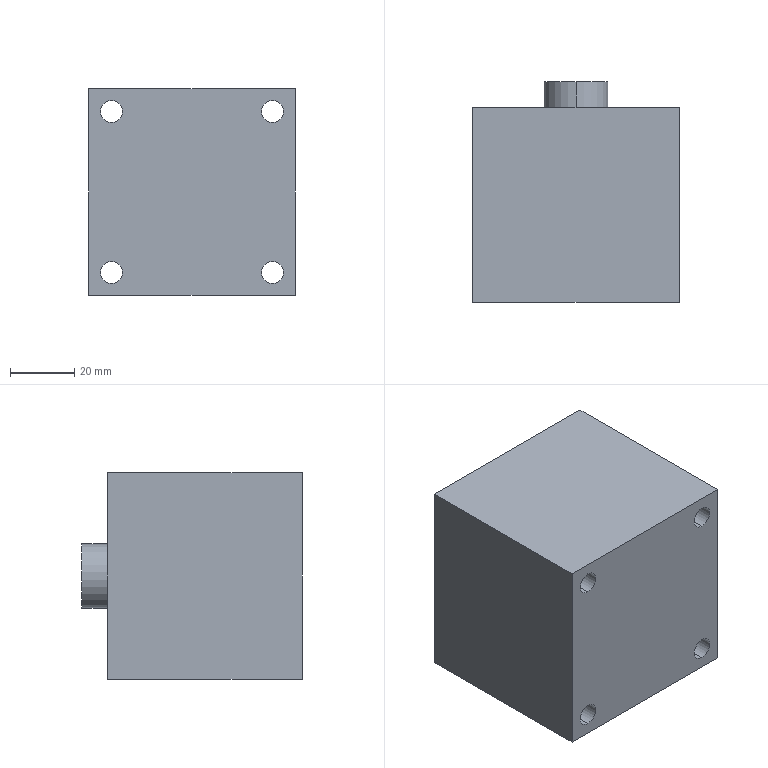Part | STEP file | 1 solid | 21 faces | box 64 x 68.5 x 64 mm | volume 240094 mm3 | cylinder 12 | plane 7 | cone 2 | commonest cylinder face diameters 6.8 x8 8.5 x2 20 x2
STEP:
#1=CARTESIAN_POINT('',(0.,0.,0.));
#2=DIRECTION('',(0.,0.,1.));
#3=DIRECTION('',(1.,0.,0.));
#4=AXIS2_PLACEMENT_3D('',#1,#2,#3);
#5=CARTESIAN_POINT('',(0.,44.,4.25));
#6=VERTEX_POINT('',#5);
#7=CARTESIAN_POINT('',(0.,68.5,4.25));
#8=VERTEX_POINT('',#7);
#9=CARTESIAN_POINT('',(0.,68.5,4.25));
#10=DIRECTION('',(0.,1.,0.));
#11=VECTOR('',#10,1.);
#12=LINE('',#9,#11);
#13=CARTESIAN_POINT('',(0.,68.5,0.));
#14=DIRECTION('',(0.,1.,0.));
#15=DIRECTION('',(0.,0.,1.));
#16=AXIS2_PLACEMENT_3D('',#13,#14,#15);
#17=CYLINDRICAL_SURFACE('',#16,4.25);
#18=CARTESIAN_POINT('',(6.283,0.));
#19=DIRECTION('',(0.,1.));
#20=VECTOR('',#19,1.);
#21=LINE('',#18,#20);
#22=(GEOMETRIC_REPRESENTATION_CONTEXT(2)PARAMETRIC_REPRESENTATION_CONTEXT()REPRESENTATION_CONTEXT('',''));
#23=DEFINITIONAL_REPRESENTATION('',(#21),#22);
#24=PCURVE('',#17,#23);
#25=CARTESIAN_POINT('',(0.,68.5,0.));
#26=DIRECTION('',(0.,1.,0.));
#27=DIRECTION('',(0.,0.,1.));
#28=AXIS2_PLACEMENT_3D('',#25,#26,#27);
#29=CYLINDRICAL_SURFACE('',#28,4.25);
#30=CARTESIAN_POINT('',(0.,0.));
#31=DIRECTION('',(0.,1.));
#32=VECTOR('',#31,1.);
#33=LINE('',#30,#32);
#34=(GEOMETRIC_REPRESENTATION_CONTEXT(2)PARAMETRIC_REPRESENTATION_CONTEXT()REPRESENTATION_CONTEXT('',''));
#35=DEFINITIONAL_REPRESENTATION('',(#33),#34);
#36=PCURVE('',#29,#35);
#37=SURFACE_CURVE('',#12,(#24,#36),.PCURVE_S1.);
#38=EDGE_CURVE('',#6,#8,#37,.T.);
#39=ORIENTED_EDGE('',*,*,#38,.T.);
#40=CARTESIAN_POINT('',(0.,68.5,-4.25));
#41=VERTEX_POINT('',#40);
#42=CARTESIAN_POINT('',(0.,68.5,0.));
#43=DIRECTION('',(0.,1.,0.));
#44=DIRECTION('',(0.,0.,1.));
#45=AXIS2_PLACEMENT_3D('',#42,#43,#44);
#46=CIRCLE('',#45,4.25);
#47=CARTESIAN_POINT('',(0.,0.));
#48=DIRECTION('',(1.,0.));
#49=VECTOR('',#48,1.);
#50=LINE('',#47,#49);
#51=(GEOMETRIC_REPRESENTATION_CONTEXT(2)PARAMETRIC_REPRESENTATION_CONTEXT()REPRESENTATION_CONTEXT('',''));
#52=DEFINITIONAL_REPRESENTATION('',(#50),#51);
#53=PCURVE('',#17,#52);
#54=CARTESIAN_POINT('',(0.,68.5,0.));
#55=DIRECTION('',(0.,1.,0.));
#56=DIRECTION('',(0.,0.,1.));
#57=AXIS2_PLACEMENT_3D('',#54,#55,#56);
#58=PLANE('',#57);
#59=CARTESIAN_POINT('',(0.,0.));
#60=DIRECTION('',(1.,0.));
#61=AXIS2_PLACEMENT_2D('',#59,#60);
#62=CIRCLE('',#61,4.25);
#63=(GEOMETRIC_REPRESENTATION_CONTEXT(2)PARAMETRIC_REPRESENTATION_CONTEXT()REPRESENTATION_CONTEXT('',''));
#64=DEFINITIONAL_REPRESENTATION('',(#62),#63);
#65=PCURVE('',#58,#64);
#66=SURFACE_CURVE('',#46,(#53,#65),.PCURVE_S1.);
#67=EDGE_CURVE('',#41,#8,#66,.T.);
#68=ORIENTED_EDGE('',*,*,#67,.F.);
#69=CARTESIAN_POINT('',(0.,44.,-4.25));
#70=VERTEX_POINT('',#69);
#71=CARTESIAN_POINT('',(0.,68.5,-4.25));
#72=DIRECTION('',(0.,1.,0.));
#73=VECTOR('',#72,1.);
#74=LINE('',#71,#73);
#75=CARTESIAN_POINT('',(3.142,0.));
#76=DIRECTION('',(0.,1.));
#77=VECTOR('',#76,1.);
#78=LINE('',#75,#77);
#79=(GEOMETRIC_REPRESENTATION_CONTEXT(2)PARAMETRIC_REPRESENTATION_CONTEXT()REPRESENTATION_CONTEXT('',''));
#80=DEFINITIONAL_REPRESENTATION('',(#78),#79);
#81=PCURVE('',#17,#80);
#82=CARTESIAN_POINT('',(3.142,0.));
#83=DIRECTION('',(0.,1.));
#84=VECTOR('',#83,1.);
#85=LINE('',#82,#84);
#86=(GEOMETRIC_REPRESENTATION_CONTEXT(2)PARAMETRIC_REPRESENTATION_CONTEXT()REPRESENTATION_CONTEXT('',''));
#87=DEFINITIONAL_REPRESENTATION('',(#85),#86);
#88=PCURVE('',#29,#87);
#89=SURFACE_CURVE('',#74,(#81,#88),.PCURVE_S1.);
#90=EDGE_CURVE('',#70,#41,#89,.T.);
#91=ORIENTED_EDGE('',*,*,#90,.F.);
#92=CARTESIAN_POINT('',(0.,44.,0.));
#93=DIRECTION('',(0.,1.,0.));
#94=DIRECTION('',(0.,0.,1.));
#95=AXIS2_PLACEMENT_3D('',#92,#93,#94);
#96=CIRCLE('',#95,4.25);
#97=CARTESIAN_POINT('',(0.,-24.5));
#98=DIRECTION('',(1.,0.));
#99=VECTOR('',#98,1.);
#100=LINE('',#97,#99);
#101=(GEOMETRIC_REPRESENTATION_CONTEXT(2)PARAMETRIC_REPRESENTATION_CONTEXT()REPRESENTATION_CONTEXT('',''));
#102=DEFINITIONAL_REPRESENTATION('',(#100),#101);
#103=PCURVE('',#17,#102);
#104=CARTESIAN_POINT('',(0.,44.,0.));
#105=DIRECTION('',(0.,1.,0.));
#106=DIRECTION('',(0.,0.,1.));
#107=AXIS2_PLACEMENT_3D('',#104,#105,#106);
#108=CONICAL_SURFACE('',#107,4.25,1.03);
#109=CARTESIAN_POINT('',(0.,0.));
#110=DIRECTION('',(1.,0.));
#111=VECTOR('',#110,1.);
#112=LINE('',#109,#111);
#113=(GEOMETRIC_REPRESENTATION_CONTEXT(2)PARAMETRIC_REPRESENTATION_CONTEXT()REPRESENTATION_CONTEXT('',''));
#114=DEFINITIONAL_REPRESENTATION('',(#112),#113);
#115=PCURVE('',#108,#114);
#116=SURFACE_CURVE('',#96,(#103,#115),.PCURVE_S1.);
#117=EDGE_CURVE('',#70,#6,#116,.T.);
#118=ORIENTED_EDGE('',*,*,#117,.T.);
#119=EDGE_LOOP('',(#39,#68,#91,#118));
#120=FACE_BOUND('',#119,.F.);
#121=ADVANCED_FACE('',(#120),#17,.F.);
#122=ORIENTED_EDGE('',*,*,#117,.F.);
#123=CARTESIAN_POINT('',(0.,41.446,0.));
#124=VERTEX_POINT('',#123);
#125=CARTESIAN_POINT('',(0.,44.,-4.25));
#126=DIRECTION('',(0.,0.515,-0.8572));
#127=VECTOR('',#126,1.);
#128=LINE('',#125,#127);
#129=CARTESIAN_POINT('',(3.142,0.));
#130=DIRECTION('',(0.,1.));
#131=VECTOR('',#130,1.);
#132=LINE('',#129,#131);
#133=(GEOMETRIC_REPRESENTATION_CONTEXT(2)PARAMETRIC_REPRESENTATION_CONTEXT()REPRESENTATION_CONTEXT('',''));
#134=DEFINITIONAL_REPRESENTATION('',(#132),#133);
#135=PCURVE('',#108,#134);
#136=CARTESIAN_POINT('',(0.,44.,0.));
#137=DIRECTION('',(0.,1.,0.));
#138=DIRECTION('',(0.,0.,1.));
#139=AXIS2_PLACEMENT_3D('',#136,#137,#138);
#140=CONICAL_SURFACE('',#139,4.25,1.03);
#141=CARTESIAN_POINT('',(3.142,0.));
#142=DIRECTION('',(0.,1.));
#143=VECTOR('',#142,1.);
#144=LINE('',#141,#143);
#145=(GEOMETRIC_REPRESENTATION_CONTEXT(2)PARAMETRIC_REPRESENTATION_CONTEXT()REPRESENTATION_CONTEXT('',''));
#146=DEFINITIONAL_REPRESENTATION('',(#144),#145);
#147=PCURVE('',#140,#146);
#148=SURFACE_CURVE('',#128,(#135,#147),.PCURVE_S1.);
#149=EDGE_CURVE('',#124,#70,#148,.T.);
#150=ORIENTED_EDGE('',*,*,#149,.F.);
#151=CARTESIAN_POINT('',(0.,44.,4.25));
#152=DIRECTION('',(0.,0.515,0.8572));
#153=VECTOR('',#152,1.);
#154=LINE('',#151,#153);
#155=CARTESIAN_POINT('',(6.283,0.));
#156=DIRECTION('',(0.,1.));
#157=VECTOR('',#156,1.);
#158=LINE('',#155,#157);
#159=(GEOMETRIC_REPRESENTATION_CONTEXT(2)PARAMETRIC_REPRESENTATION_CONTEXT()REPRESENTATION_CONTEXT('',''));
#160=DEFINITIONAL_REPRESENTATION('',(#158),#159);
#161=PCURVE('',#108,#160);
#162=CARTESIAN_POINT('',(0.,0.));
#163=DIRECTION('',(0.,1.));
#164=VECTOR('',#163,1.);
#165=LINE('',#162,#164);
#166=(GEOMETRIC_REPRESENTATION_CONTEXT(2)PARAMETRIC_REPRESENTATION_CONTEXT()REPRESENTATION_CONTEXT('',''));
#167=DEFINITIONAL_REPRESENTATION('',(#165),#166);
#168=PCURVE('',#140,#167);
#169=SURFACE_CURVE('',#154,(#161,#168),.PCURVE_S1.);
#170=EDGE_CURVE('',#124,#6,#169,.T.);
#171=ORIENTED_EDGE('',*,*,#170,.T.);
#172=EDGE_LOOP('',(#122,#150,#171));
#173=FACE_BOUND('',#172,.F.);
#174=ADVANCED_FACE('',(#173),#108,.F.);
#175=CARTESIAN_POINT('',(25.,0.,-21.6));
#176=VERTEX_POINT('',#175);
#177=CARTESIAN_POINT('',(25.,60.5,-21.6));
#178=VERTEX_POINT('',#177);
#179=CARTESIAN_POINT('',(25.,60.5,-21.6));
#180=DIRECTION('',(0.,1.,0.));
#181=VECTOR('',#180,1.);
#182=LINE('',#179,#181);
#183=CARTESIAN_POINT('',(25.,60.5,-25.));
#184=DIRECTION('',(0.,1.,0.));
#185=DIRECTION('',(0.,0.,1.));
#186=AXIS2_PLACEMENT_3D('',#183,#184,#185);
#187=CYLINDRICAL_SURFACE('',#186,3.4);
#188=CARTESIAN_POINT('',(6.283,0.));
#189=DIRECTION('',(0.,1.));
#190=VECTOR('',#189,1.);
#191=LINE('',#188,#190);
#192=(GEOMETRIC_REPRESENTATION_CONTEXT(2)PARAMETRIC_REPRESENTATION_CONTEXT()REPRESENTATION_CONTEXT('',''));
#193=DEFINITIONAL_REPRESENTATION('',(#191),#192);
#194=PCURVE('',#187,#193);
#195=CARTESIAN_POINT('',(25.,60.5,-25.));
#196=DIRECTION('',(0.,1.,0.));
#197=DIRECTION('',(0.,0.,1.));
#198=AXIS2_PLACEMENT_3D('',#195,#196,#197);
#199=CYLINDRICAL_SURFACE('',#198,3.4);
#200=CARTESIAN_POINT('',(0.,0.));
#201=DIRECTION('',(0.,1.));
#202=VECTOR('',#201,1.);
#203=LINE('',#200,#202);
#204=(GEOMETRIC_REPRESENTATION_CONTEXT(2)PARAMETRIC_REPRESENTATION_CONTEXT()REPRESENTATION_CONTEXT('',''));
#205=DEFINITIONAL_REPRESENTATION('',(#203),#204);
#206=PCURVE('',#199,#205);
#207=SURFACE_CURVE('',#182,(#194,#206),.PCURVE_S1.);
#208=EDGE_CURVE('',#176,#178,#207,.T.);
#209=ORIENTED_EDGE('',*,*,#208,.T.);
#210=CARTESIAN_POINT('',(25.,60.5,-28.4));
#211=VERTEX_POINT('',#210);
#212=CARTESIAN_POINT('',(25.,60.5,-25.));
#213=DIRECTION('',(0.,1.,0.));
#214=DIRECTION('',(0.,0.,1.));
#215=AXIS2_PLACEMENT_3D('',#212,#213,#214);
#216=CIRCLE('',#215,3.4);
#217=CARTESIAN_POINT('',(0.,0.));
#218=DIRECTION('',(1.,0.));
#219=VECTOR('',#218,1.);
#220=LINE('',#217,#219);
#221=(GEOMETRIC_REPRESENTATION_CONTEXT(2)PARAMETRIC_REPRESENTATION_CONTEXT()REPRESENTATION_CONTEXT('',''));
#222=DEFINITIONAL_REPRESENTATION('',(#220),#221);
#223=PCURVE('',#187,#222);
#224=CARTESIAN_POINT('',(0.,60.5,0.));
#225=DIRECTION('',(0.,1.,0.));
#226=DIRECTION('',(0.,0.,1.));
#227=AXIS2_PLACEMENT_3D('',#224,#225,#226);
#228=PLANE('',#227);
#229=CARTESIAN_POINT('',(-25.,25.));
#230=DIRECTION('',(1.,0.));
#231=AXIS2_PLACEMENT_2D('',#229,#230);
#232=CIRCLE('',#231,3.4);
#233=(GEOMETRIC_REPRESENTATION_CONTEXT(2)PARAMETRIC_REPRESENTATION_CONTEXT()REPRESENTATION_CONTEXT('',''));
#234=DEFINITIONAL_REPRESENTATION('',(#232),#233);
#235=PCURVE('',#228,#234);
#236=SURFACE_CURVE('',#216,(#223,#235),.PCURVE_S1.);
#237=EDGE_CURVE('',#211,#178,#236,.T.);
#238=ORIENTED_EDGE('',*,*,#237,.F.);
#239=CARTESIAN_POINT('',(25.,0.,-28.4));
#240=VERTEX_POINT('',#239);
#241=CARTESIAN_POINT('',(25.,60.5,-28.4));
#242=DIRECTION('',(0.,1.,0.));
#243=VECTOR('',#242,1.);
#244=LINE('',#241,#243);
#245=CARTESIAN_POINT('',(3.142,0.));
#246=DIRECTION('',(0.,1.));
#247=VECTOR('',#246,1.);
#248=LINE('',#245,#247);
#249=(GEOMETRIC_REPRESENTATION_CONTEXT(2)PARAMETRIC_REPRESENTATION_CONTEXT()REPRESENTATION_CONTEXT('',''));
#250=DEFINITIONAL_REPRESENTATION('',(#248),#249);
#251=PCURVE('',#187,#250);
#252=CARTESIAN_POINT('',(3.142,0.));
#253=DIRECTION('',(0.,1.));
#254=VECTOR('',#253,1.);
#255=LINE('',#252,#254);
#256=(GEOMETRIC_REPRESENTATION_CONTEXT(2)PARAMETRIC_REPRESENTATION_CONTEXT()REPRESENTATION_CONTEXT('',''));
#257=DEFINITIONAL_REPRESENTATION('',(#255),#256);
#258=PCURVE('',#199,#257);
#259=SURFACE_CURVE('',#244,(#251,#258),.PCURVE_S1.);
#260=EDGE_CURVE('',#240,#211,#259,.T.);
#261=ORIENTED_EDGE('',*,*,#260,.F.);
#262=CARTESIAN_POINT('',(25.,0.,-25.));
#263=DIRECTION('',(0.,1.,0.));
#264=DIRECTION('',(0.,0.,1.));
#265=AXIS2_PLACEMENT_3D('',#262,#263,#264);
#266=CIRCLE('',#265,3.4);
#267=CARTESIAN_POINT('',(0.,-60.5));
#268=DIRECTION('',(1.,0.));
#269=VECTOR('',#268,1.);
#270=LINE('',#267,#269);
#271=(GEOMETRIC_REPRESENTATION_CONTEXT(2)PARAMETRIC_REPRESENTATION_CONTEXT()REPRESENTATION_CONTEXT('',''));
#272=DEFINITIONAL_REPRESENTATION('',(#270),#271);
#273=PCURVE('',#187,#272);
#274=CARTESIAN_POINT('',(0.,0.,0.));
#275=DIRECTION('',(0.,1.,0.));
#276=DIRECTION('',(0.,0.,1.));
#277=AXIS2_PLACEMENT_3D('',#274,#275,#276);
#278=PLANE('',#277);
#279=CARTESIAN_POINT('',(-25.,25.));
#280=DIRECTION('',(1.,0.));
#281=AXIS2_PLACEMENT_2D('',#279,#280);
#282=CIRCLE('',#281,3.4);
#283=(GEOMETRIC_REPRESENTATION_CONTEXT(2)PARAMETRIC_REPRESENTATION_CONTEXT()REPRESENTATION_CONTEXT('',''));
#284=DEFINITIONAL_REPRESENTATION('',(#282),#283);
#285=PCURVE('',#278,#284);
#286=SURFACE_CURVE('',#266,(#273,#285),.PCURVE_S1.);
#287=EDGE_CURVE('',#240,#176,#286,.T.);
#288=ORIENTED_EDGE('',*,*,#287,.T.);
#289=EDGE_LOOP('',(#209,#238,#261,#288));
#290=FACE_BOUND('',#289,.F.);
#291=ADVANCED_FACE('',(#290),#187,.F.);
#292=CARTESIAN_POINT('',(25.,0.,28.4));
#293=VERTEX_POINT('',#292);
#294=CARTESIAN_POINT('',(25.,60.5,28.4));
#295=VERTEX_POINT('',#294);
#296=CARTESIAN_POINT('',(25.,60.5,28.4));
#297=DIRECTION('',(0.,1.,0.));
#298=VECTOR('',#297,1.);
#299=LINE('',#296,#298);
#300=CARTESIAN_POINT('',(25.,60.5,25.));
#301=DIRECTION('',(0.,1.,0.));
#302=DIRECTION('',(0.,0.,1.));
#303=AXIS2_PLACEMENT_3D('',#300,#301,#302);
#304=CYLINDRICAL_SURFACE('',#303,3.4);
#305=CARTESIAN_POINT('',(6.283,0.));
#306=DIRECTION('',(0.,1.));
#307=VECTOR('',#306,1.);
#308=LINE('',#305,#307);
#309=(GEOMETRIC_REPRESENTATION_CONTEXT(2)PARAMETRIC_REPRESENTATION_CONTEXT()REPRESENTATION_CONTEXT('',''));
#310=DEFINITIONAL_REPRESENTATION('',(#308),#309);
#311=PCURVE('',#304,#310);
#312=CARTESIAN_POINT('',(25.,60.5,25.));
#313=DIRECTION('',(0.,1.,0.));
#314=DIRECTION('',(0.,0.,1.));
#315=AXIS2_PLACEMENT_3D('',#312,#313,#314);
#316=CYLINDRICAL_SURFACE('',#315,3.4);
#317=CARTESIAN_POINT('',(0.,0.));
#318=DIRECTION('',(0.,1.));
#319=VECTOR('',#318,1.);
#320=LINE('',#317,#319);
#321=(GEOMETRIC_REPRESENTATION_CONTEXT(2)PARAMETRIC_REPRESENTATION_CONTEXT()REPRESENTATION_CONTEXT('',''));
#322=DEFINITIONAL_REPRESENTATION('',(#320),#321);
#323=PCURVE('',#316,#322);
#324=SURFACE_CURVE('',#299,(#311,#323),.PCURVE_S1.);
#325=EDGE_CURVE('',#293,#295,#324,.T.);
#326=ORIENTED_EDGE('',*,*,#325,.T.);
#327=CARTESIAN_POINT('',(25.,60.5,21.6));
#328=VERTEX_POINT('',#327);
#329=CARTESIAN_POINT('',(25.,60.5,25.));
#330=DIRECTION('',(0.,1.,0.));
#331=DIRECTION('',(0.,0.,1.));
#332=AXIS2_PLACEMENT_3D('',#329,#330,#331);
#333=CIRCLE('',#332,3.4);
#334=CARTESIAN_POINT('',(0.,0.));
#335=DIRECTION('',(1.,0.));
#336=VECTOR('',#335,1.);
#337=LINE('',#334,#336);
#338=(GEOMETRIC_REPRESENTATION_CONTEXT(2)PARAMETRIC_REPRESENTATION_CONTEXT()REPRESENTATION_CONTEXT('',''));
#339=DEFINITIONAL_REPRESENTATION('',(#337),#338);
#340=PCURVE('',#304,#339);
#341=CARTESIAN_POINT('',(25.,25.));
#342=DIRECTION('',(1.,0.));
#343=AXIS2_PLACEMENT_2D('',#341,#342);
#344=CIRCLE('',#343,3.4);
#345=(GEOMETRIC_REPRESENTATION_CONTEXT(2)PARAMETRIC_REPRESENTATION_CONTEXT()REPRESENTATION_CONTEXT('',''));
#346=DEFINITIONAL_REPRESENTATION('',(#344),#345);
#347=PCURVE('',#228,#346);
#348=SURFACE_CURVE('',#333,(#340,#347),.PCURVE_S1.);
#349=EDGE_CURVE('',#328,#295,#348,.T.);
#350=ORIENTED_EDGE('',*,*,#349,.F.);
#351=CARTESIAN_POINT('',(25.,0.,21.6));
#352=VERTEX_POINT('',#351);
#353=CARTESIAN_POINT('',(25.,60.5,21.6));
#354=DIRECTION('',(0.,1.,0.));
#355=VECTOR('',#354,1.);
#356=LINE('',#353,#355);
#357=CARTESIAN_POINT('',(3.142,0.));
#358=DIRECTION('',(0.,1.));
#359=VECTOR('',#358,1.);
#360=LINE('',#357,#359);
#361=(GEOMETRIC_REPRESENTATION_CONTEXT(2)PARAMETRIC_REPRESENTATION_CONTEXT()REPRESENTATION_CONTEXT('',''));
#362=DEFINITIONAL_REPRESENTATION('',(#360),#361);
#363=PCURVE('',#304,#362);
#364=CARTESIAN_POINT('',(3.142,0.));
#365=DIRECTION('',(0.,1.));
#366=VECTOR('',#365,1.);
#367=LINE('',#364,#366);
#368=(GEOMETRIC_REPRESENTATION_CONTEXT(2)PARAMETRIC_REPRESENTATION_CONTEXT()REPRESENTATION_CONTEXT('',''));
#369=DEFINITIONAL_REPRESENTATION('',(#367),#368);
#370=PCURVE('',#316,#369);
#371=SURFACE_CURVE('',#356,(#363,#370),.PCURVE_S1.);
#372=EDGE_CURVE('',#352,#328,#371,.T.);
#373=ORIENTED_EDGE('',*,*,#372,.F.);
#374=CARTESIAN_POINT('',(25.,0.,25.));
#375=DIRECTION('',(0.,1.,0.));
#376=DIRECTION('',(0.,0.,1.));
#377=AXIS2_PLACEMENT_3D('',#374,#375,#376);
#378=CIRCLE('',#377,3.4);
#379=CARTESIAN_POINT('',(0.,-60.5));
#380=DIRECTION('',(1.,0.));
#381=VECTOR('',#380,1.);
#382=LINE('',#379,#381);
#383=(GEOMETRIC_REPRESENTATION_CONTEXT(2)PARAMETRIC_REPRESENTATION_CONTEXT()REPRESENTATION_CONTEXT('',''));
#384=DEFINITIONAL_REPRESENTATION('',(#382),#383);
#385=PCURVE('',#304,#384);
#386=CARTESIAN_POINT('',(25.,25.));
#387=DIRECTION('',(1.,0.));
#388=AXIS2_PLACEMENT_2D('',#386,#387);
#389=CIRCLE('',#388,3.4);
#390=(GEOMETRIC_REPRESENTATION_CONTEXT(2)PARAMETRIC_REPRESENTATION_CONTEXT()REPRESENTATION_CONTEXT('',''));
#391=DEFINITIONAL_REPRESENTATION('',(#389),#390);
#392=PCURVE('',#278,#391);
#393=SURFACE_CURVE('',#378,(#385,#392),.PCURVE_S1.);
#394=EDGE_CURVE('',#352,#293,#393,.T.);
#395=ORIENTED_EDGE('',*,*,#394,.T.);
#396=EDGE_LOOP('',(#326,#350,#373,#395));
#397=FACE_BOUND('',#396,.F.);
#398=ADVANCED_FACE('',(#397),#304,.F.);
#399=CARTESIAN_POINT('',(-25.,0.,28.4));
#400=VERTEX_POINT('',#399);
#401=CARTESIAN_POINT('',(-25.,60.5,28.4));
#402=VERTEX_POINT('',#401);
#403=CARTESIAN_POINT('',(-25.,60.5,28.4));
#404=DIRECTION('',(0.,1.,0.));
#405=VECTOR('',#404,1.);
#406=LINE('',#403,#405);
#407=CARTESIAN_POINT('',(-25.,60.5,25.));
#408=DIRECTION('',(0.,1.,0.));
#409=DIRECTION('',(0.,0.,1.));
#410=AXIS2_PLACEMENT_3D('',#407,#408,#409);
#411=CYLINDRICAL_SURFACE('',#410,3.4);
#412=CARTESIAN_POINT('',(6.283,0.));
#413=DIRECTION('',(0.,1.));
#414=VECTOR('',#413,1.);
#415=LINE('',#412,#414);
#416=(GEOMETRIC_REPRESENTATION_CONTEXT(2)PARAMETRIC_REPRESENTATION_CONTEXT()REPRESENTATION_CONTEXT('',''));
#417=DEFINITIONAL_REPRESENTATION('',(#415),#416);
#418=PCURVE('',#411,#417);
#419=CARTESIAN_POINT('',(-25.,60.5,25.));
#420=DIRECTION('',(0.,1.,0.));
#421=DIRECTION('',(0.,0.,1.));
#422=AXIS2_PLACEMENT_3D('',#419,#420,#421);
#423=CYLINDRICAL_SURFACE('',#422,3.4);
#424=CARTESIAN_POINT('',(0.,0.));
#425=DIRECTION('',(0.,1.));
#426=VECTOR('',#425,1.);
#427=LINE('',#424,#426);
#428=(GEOMETRIC_REPRESENTATION_CONTEXT(2)PARAMETRIC_REPRESENTATION_CONTEXT()REPRESENTATION_CONTEXT('',''));
#429=DEFINITIONAL_REPRESENTATION('',(#427),#428);
#430=PCURVE('',#423,#429);
#431=SURFACE_CURVE('',#406,(#418,#430),.PCURVE_S1.);
#432=EDGE_CURVE('',#400,#402,#431,.T.);
#433=ORIENTED_EDGE('',*,*,#432,.T.);
#434=CARTESIAN_POINT('',(-25.,60.5,21.6));
#435=VERTEX_POINT('',#434);
#436=CARTESIAN_POINT('',(-25.,60.5,25.));
#437=DIRECTION('',(0.,1.,0.));
#438=DIRECTION('',(0.,0.,1.));
#439=AXIS2_PLACEMENT_3D('',#436,#437,#438);
#440=CIRCLE('',#439,3.4);
#441=CARTESIAN_POINT('',(0.,0.));
#442=DIRECTION('',(1.,0.));
#443=VECTOR('',#442,1.);
#444=LINE('',#441,#443);
#445=(GEOMETRIC_REPRESENTATION_CONTEXT(2)PARAMETRIC_REPRESENTATION_CONTEXT()REPRESENTATION_CONTEXT('',''));
#446=DEFINITIONAL_REPRESENTATION('',(#444),#445);
#447=PCURVE('',#411,#446);
#448=CARTESIAN_POINT('',(25.,-25.));
#449=DIRECTION('',(1.,0.));
#450=AXIS2_PLACEMENT_2D('',#448,#449);
#451=CIRCLE('',#450,3.4);
#452=(GEOMETRIC_REPRESENTATION_CONTEXT(2)PARAMETRIC_REPRESENTATION_CONTEXT()REPRESENTATION_CONTEXT('',''));
#453=DEFINITIONAL_REPRESENTATION('',(#451),#452);
#454=PCURVE('',#228,#453);
#455=SURFACE_CURVE('',#440,(#447,#454),.PCURVE_S1.);
#456=EDGE_CURVE('',#435,#402,#455,.T.);
#457=ORIENTED_EDGE('',*,*,#456,.F.);
#458=CARTESIAN_POINT('',(-25.,0.,21.6));
#459=VERTEX_POINT('',#458);
#460=CARTESIAN_POINT('',(-25.,60.5,21.6));
#461=DIRECTION('',(0.,1.,0.));
#462=VECTOR('',#461,1.);
#463=LINE('',#460,#462);
#464=CARTESIAN_POINT('',(3.142,0.));
#465=DIRECTION('',(0.,1.));
#466=VECTOR('',#465,1.);
#467=LINE('',#464,#466);
#468=(GEOMETRIC_REPRESENTATION_CONTEXT(2)PARAMETRIC_REPRESENTATION_CONTEXT()REPRESENTATION_CONTEXT('',''));
#469=DEFINITIONAL_REPRESENTATION('',(#467),#468);
#470=PCURVE('',#411,#469);
#471=CARTESIAN_POINT('',(3.142,0.));
#472=DIRECTION('',(0.,1.));
#473=VECTOR('',#472,1.);
#474=LINE('',#471,#473);
#475=(GEOMETRIC_REPRESENTATION_CONTEXT(2)PARAMETRIC_REPRESENTATION_CONTEXT()REPRESENTATION_CONTEXT('',''));
#476=DEFINITIONAL_REPRESENTATION('',(#474),#475);
#477=PCURVE('',#423,#476);
#478=SURFACE_CURVE('',#463,(#470,#477),.PCURVE_S1.);
#479=EDGE_CURVE('',#459,#435,#478,.T.);
#480=ORIENTED_EDGE('',*,*,#479,.F.);
#481=CARTESIAN_POINT('',(-25.,0.,25.));
#482=DIRECTION('',(0.,1.,0.));
#483=DIRECTION('',(0.,0.,1.));
#484=AXIS2_PLACEMENT_3D('',#481,#482,#483);
#485=CIRCLE('',#484,3.4);
#486=CARTESIAN_POINT('',(0.,-60.5));
#487=DIRECTION('',(1.,0.));
#488=VECTOR('',#487,1.);
#489=LINE('',#486,#488);
#490=(GEOMETRIC_REPRESENTATION_CONTEXT(2)PARAMETRIC_REPRESENTATION_CONTEXT()REPRESENTATION_CONTEXT('',''));
#491=DEFINITIONAL_REPRESENTATION('',(#489),#490);
#492=PCURVE('',#411,#491);
#493=CARTESIAN_POINT('',(25.,-25.));
#494=DIRECTION('',(1.,0.));
#495=AXIS2_PLACEMENT_2D('',#493,#494);
#496=CIRCLE('',#495,3.4);
#497=(GEOMETRIC_REPRESENTATION_CONTEXT(2)PARAMETRIC_REPRESENTATION_CONTEXT()REPRESENTATION_CONTEXT('',''));
#498=DEFINITIONAL_REPRESENTATION('',(#496),#497);
#499=PCURVE('',#278,#498);
#500=SURFACE_CURVE('',#485,(#492,#499),.PCURVE_S1.);
#501=EDGE_CURVE('',#459,#400,#500,.T.);
#502=ORIENTED_EDGE('',*,*,#501,.T.);
#503=EDGE_LOOP('',(#433,#457,#480,#502));
#504=FACE_BOUND('',#503,.F.);
#505=ADVANCED_FACE('',(#504),#411,.F.);
#506=CARTESIAN_POINT('',(-25.,0.,-21.6));
#507=VERTEX_POINT('',#506);
#508=CARTESIAN_POINT('',(-25.,60.5,-21.6));
#509=VERTEX_POINT('',#508);
#510=CARTESIAN_POINT('',(-25.,60.5,-21.6));
#511=DIRECTION('',(0.,1.,0.));
#512=VECTOR('',#511,1.);
#513=LINE('',#510,#512);
#514=CARTESIAN_POINT('',(-25.,60.5,-25.));
#515=DIRECTION('',(0.,1.,0.));
#516=DIRECTION('',(0.,0.,1.));
#517=AXIS2_PLACEMENT_3D('',#514,#515,#516);
#518=CYLINDRICAL_SURFACE('',#517,3.4);
#519=CARTESIAN_POINT('',(6.283,0.));
#520=DIRECTION('',(0.,1.));
#521=VECTOR('',#520,1.);
#522=LINE('',#519,#521);
#523=(GEOMETRIC_REPRESENTATION_CONTEXT(2)PARAMETRIC_REPRESENTATION_CONTEXT()REPRESENTATION_CONTEXT('',''));
#524=DEFINITIONAL_REPRESENTATION('',(#522),#523);
#525=PCURVE('',#518,#524);
#526=CARTESIAN_POINT('',(-25.,60.5,-25.));
#527=DIRECTION('',(0.,1.,0.));
#528=DIRECTION('',(0.,0.,1.));
#529=AXIS2_PLACEMENT_3D('',#526,#527,#528);
#530=CYLINDRICAL_SURFACE('',#529,3.4);
#531=CARTESIAN_POINT('',(0.,0.));
#532=DIRECTION('',(0.,1.));
#533=VECTOR('',#532,1.);
#534=LINE('',#531,#533);
#535=(GEOMETRIC_REPRESENTATION_CONTEXT(2)PARAMETRIC_REPRESENTATION_CONTEXT()REPRESENTATION_CONTEXT('',''));
#536=DEFINITIONAL_REPRESENTATION('',(#534),#535);
#537=PCURVE('',#530,#536);
#538=SURFACE_CURVE('',#513,(#525,#537),.PCURVE_S1.);
#539=EDGE_CURVE('',#507,#509,#538,.T.);
#540=ORIENTED_EDGE('',*,*,#539,.T.);
#541=CARTESIAN_POINT('',(-25.,60.5,-28.4));
#542=VERTEX_POINT('',#541);
#543=CARTESIAN_POINT('',(-25.,60.5,-25.));
#544=DIRECTION('',(0.,1.,0.));
#545=DIRECTION('',(0.,0.,1.));
#546=AXIS2_PLACEMENT_3D('',#543,#544,#545);
#547=CIRCLE('',#546,3.4);
#548=CARTESIAN_POINT('',(0.,0.));
#549=DIRECTION('',(1.,0.));
#550=VECTOR('',#549,1.);
#551=LINE('',#548,#550);
#552=(GEOMETRIC_REPRESENTATION_CONTEXT(2)PARAMETRIC_REPRESENTATION_CONTEXT()REPRESENTATION_CONTEXT('',''));
#553=DEFINITIONAL_REPRESENTATION('',(#551),#552);
#554=PCURVE('',#518,#553);
#555=CARTESIAN_POINT('',(-25.,-25.));
#556=DIRECTION('',(1.,0.));
#557=AXIS2_PLACEMENT_2D('',#555,#556);
#558=CIRCLE('',#557,3.4);
#559=(GEOMETRIC_REPRESENTATION_CONTEXT(2)PARAMETRIC_REPRESENTATION_CONTEXT()REPRESENTATION_CONTEXT('',''));
#560=DEFINITIONAL_REPRESENTATION('',(#558),#559);
#561=PCURVE('',#228,#560);
#562=SURFACE_CURVE('',#547,(#554,#561),.PCURVE_S1.);
#563=EDGE_CURVE('',#542,#509,#562,.T.);
#564=ORIENTED_EDGE('',*,*,#563,.F.);
#565=CARTESIAN_POINT('',(-25.,0.,-28.4));
#566=VERTEX_POINT('',#565);
#567=CARTESIAN_POINT('',(-25.,60.5,-28.4));
#568=DIRECTION('',(0.,1.,0.));
#569=VECTOR('',#568,1.);
#570=LINE('',#567,#569);
#571=CARTESIAN_POINT('',(3.142,0.));
#572=DIRECTION('',(0.,1.));
#573=VECTOR('',#572,1.);
#574=LINE('',#571,#573);
#575=(GEOMETRIC_REPRESENTATION_CONTEXT(2)PARAMETRIC_REPRESENTATION_CONTEXT()REPRESENTATION_CONTEXT('',''));
#576=DEFINITIONAL_REPRESENTATION('',(#574),#575);
#577=PCURVE('',#518,#576);
#578=CARTESIAN_POINT('',(3.142,0.));
#579=DIRECTION('',(0.,1.));
#580=VECTOR('',#579,1.);
#581=LINE('',#578,#580);
#582=(GEOMETRIC_REPRESENTATION_CONTEXT(2)PARAMETRIC_REPRESENTATION_CONTEXT()REPRESENTATION_CONTEXT('',''));
#583=DEFINITIONAL_REPRESENTATION('',(#581),#582);
#584=PCURVE('',#530,#583);
#585=SURFACE_CURVE('',#570,(#577,#584),.PCURVE_S1.);
#586=EDGE_CURVE('',#566,#542,#585,.T.);
#587=ORIENTED_EDGE('',*,*,#586,.F.);
#588=CARTESIAN_POINT('',(-25.,0.,-25.));
#589=DIRECTION('',(0.,1.,0.));
#590=DIRECTION('',(0.,0.,1.));
#591=AXIS2_PLACEMENT_3D('',#588,#589,#590);
#592=CIRCLE('',#591,3.4);
#593=CARTESIAN_POINT('',(0.,-60.5));
#594=DIRECTION('',(1.,0.));
#595=VECTOR('',#594,1.);
#596=LINE('',#593,#595);
#597=(GEOMETRIC_REPRESENTATION_CONTEXT(2)PARAMETRIC_REPRESENTATION_CONTEXT()REPRESENTATION_CONTEXT('',''));
#598=DEFINITIONAL_REPRESENTATION('',(#596),#597);
#599=PCURVE('',#518,#598);
#600=CARTESIAN_POINT('',(-25.,-25.));
#601=DIRECTION('',(1.,0.));
#602=AXIS2_PLACEMENT_2D('',#600,#601);
#603=CIRCLE('',#602,3.4);
#604=(GEOMETRIC_REPRESENTATION_CONTEXT(2)PARAMETRIC_REPRESENTATION_CONTEXT()REPRESENTATION_CONTEXT('',''));
#605=DEFINITIONAL_REPRESENTATION('',(#603),#604);
#606=PCURVE('',#278,#605);
#607=SURFACE_CURVE('',#592,(#599,#606),.PCURVE_S1.);
#608=EDGE_CURVE('',#566,#507,#607,.T.);
#609=ORIENTED_EDGE('',*,*,#608,.T.);
#610=EDGE_LOOP('',(#540,#564,#587,#609));
#611=FACE_BOUND('',#610,.F.);
#612=ADVANCED_FACE('',(#611),#518,.F.);
#613=CARTESIAN_POINT('',(0.,68.5,10.));
#614=VERTEX_POINT('',#613);
#615=CARTESIAN_POINT('',(0.,68.5,-10.));
#616=VERTEX_POINT('',#615);
#617=CARTESIAN_POINT('',(0.,68.5,0.));
#618=DIRECTION('',(0.,1.,0.));
#619=DIRECTION('',(0.,0.,1.));
#620=AXIS2_PLACEMENT_3D('',#617,#618,#619);
#621=CIRCLE('',#620,10.);
#622=CARTESIAN_POINT('',(0.,68.5,0.));
#623=DIRECTION('',(0.,-1.,0.));
#624=DIRECTION('',(0.,0.,-1.));
#625=AXIS2_PLACEMENT_3D('',#622,#623,#624);
#626=CYLINDRICAL_SURFACE('',#625,10.);
#627=CARTESIAN_POINT('',(3.142,0.));
#628=DIRECTION('',(-1.,0.));
#629=VECTOR('',#628,1.);
#630=LINE('',#627,#629);
#631=(GEOMETRIC_REPRESENTATION_CONTEXT(2)PARAMETRIC_REPRESENTATION_CONTEXT()REPRESENTATION_CONTEXT('',''));
#632=DEFINITIONAL_REPRESENTATION('',(#630),#631);
#633=PCURVE('',#626,#632);
#634=CARTESIAN_POINT('',(0.,0.));
#635=DIRECTION('',(1.,0.));
#636=AXIS2_PLACEMENT_2D('',#634,#635);
#637=CIRCLE('',#636,10.);
#638=(GEOMETRIC_REPRESENTATION_CONTEXT(2)PARAMETRIC_REPRESENTATION_CONTEXT()REPRESENTATION_CONTEXT('',''));
#639=DEFINITIONAL_REPRESENTATION('',(#637),#638);
#640=PCURVE('',#58,#639);
#641=SURFACE_CURVE('',#621,(#633,#640),.PCURVE_S1.);
#642=EDGE_CURVE('',#614,#616,#641,.T.);
#643=ORIENTED_EDGE('',*,*,#642,.F.);
#644=CARTESIAN_POINT('',(0.,60.5,10.));
#645=VERTEX_POINT('',#644);
#646=CARTESIAN_POINT('',(0.,68.5,10.));
#647=DIRECTION('',(0.,-1.,0.));
#648=VECTOR('',#647,1.);
#649=LINE('',#646,#648);
#650=CARTESIAN_POINT('',(3.142,0.));
#651=DIRECTION('',(0.,1.));
#652=VECTOR('',#651,1.);
#653=LINE('',#650,#652);
#654=(GEOMETRIC_REPRESENTATION_CONTEXT(2)PARAMETRIC_REPRESENTATION_CONTEXT()REPRESENTATION_CONTEXT('',''));
#655=DEFINITIONAL_REPRESENTATION('',(#653),#654);
#656=PCURVE('',#626,#655);
#657=CARTESIAN_POINT('',(0.,68.5,0.));
#658=DIRECTION('',(0.,-1.,0.));
#659=DIRECTION('',(0.,0.,-1.));
#660=AXIS2_PLACEMENT_3D('',#657,#658,#659);
#661=CYLINDRICAL_SURFACE('',#660,10.);
#662=CARTESIAN_POINT('',(3.142,0.));
#663=DIRECTION('',(0.,1.));
#664=VECTOR('',#663,1.);
#665=LINE('',#662,#664);
#666=(GEOMETRIC_REPRESENTATION_CONTEXT(2)PARAMETRIC_REPRESENTATION_CONTEXT()REPRESENTATION_CONTEXT('',''));
#667=DEFINITIONAL_REPRESENTATION('',(#665),#666);
#668=PCURVE('',#661,#667);
#669=SURFACE_CURVE('',#649,(#656,#668),.PCURVE_S1.);
#670=EDGE_CURVE('',#614,#645,#669,.T.);
#671=ORIENTED_EDGE('',*,*,#670,.T.);
#672=CARTESIAN_POINT('',(0.,60.5,-10.));
#673=VERTEX_POINT('',#672);
#674=CARTESIAN_POINT('',(0.,60.5,0.));
#675=DIRECTION('',(0.,1.,0.));
#676=DIRECTION('',(0.,0.,1.));
#677=AXIS2_PLACEMENT_3D('',#674,#675,#676);
#678=CIRCLE('',#677,10.);
#679=CARTESIAN_POINT('',(3.142,8.));
#680=DIRECTION('',(-1.,0.));
#681=VECTOR('',#680,1.);
#682=LINE('',#679,#681);
#683=(GEOMETRIC_REPRESENTATION_CONTEXT(2)PARAMETRIC_REPRESENTATION_CONTEXT()REPRESENTATION_CONTEXT('',''));
#684=DEFINITIONAL_REPRESENTATION('',(#682),#683);
#685=PCURVE('',#626,#684);
#686=CARTESIAN_POINT('',(0.,0.));
#687=DIRECTION('',(1.,0.));
#688=AXIS2_PLACEMENT_2D('',#686,#687);
#689=CIRCLE('',#688,10.);
#690=(GEOMETRIC_REPRESENTATION_CONTEXT(2)PARAMETRIC_REPRESENTATION_CONTEXT()REPRESENTATION_CONTEXT('',''));
#691=DEFINITIONAL_REPRESENTATION('',(#689),#690);
#692=PCURVE('',#228,#691);
#693=SURFACE_CURVE('',#678,(#685,#692),.PCURVE_S1.);
#694=EDGE_CURVE('',#645,#673,#693,.T.);
#695=ORIENTED_EDGE('',*,*,#694,.T.);
#696=CARTESIAN_POINT('',(0.,68.5,-10.));
#697=DIRECTION('',(0.,-1.,0.));
#698=VECTOR('',#697,1.);
#699=LINE('',#696,#698);
#700=CARTESIAN_POINT('',(0.,0.));
#701=DIRECTION('',(0.,1.));
#702=VECTOR('',#701,1.);
#703=LINE('',#700,#702);
#704=(GEOMETRIC_REPRESENTATION_CONTEXT(2)PARAMETRIC_REPRESENTATION_CONTEXT()REPRESENTATION_CONTEXT('',''));
#705=DEFINITIONAL_REPRESENTATION('',(#703),#704);
#706=PCURVE('',#626,#705);
#707=CARTESIAN_POINT('',(6.283,0.));
#708=DIRECTION('',(0.,1.));
#709=VECTOR('',#708,1.);
#710=LINE('',#707,#709);
#711=(GEOMETRIC_REPRESENTATION_CONTEXT(2)PARAMETRIC_REPRESENTATION_CONTEXT()REPRESENTATION_CONTEXT('',''));
#712=DEFINITIONAL_REPRESENTATION('',(#710),#711);
#713=PCURVE('',#661,#712);
#714=SURFACE_CURVE('',#699,(#706,#713),.PCURVE_S1.);
#715=EDGE_CURVE('',#616,#673,#714,.T.);
#716=ORIENTED_EDGE('',*,*,#715,.F.);
#717=EDGE_LOOP('',(#643,#671,#695,#716));
#718=FACE_BOUND('',#717,.T.);
#719=ADVANCED_FACE('',(#718),#626,.T.);
#720=CARTESIAN_POINT('',(25.,60.5,-25.));
#721=DIRECTION('',(0.,1.,0.));
#722=DIRECTION('',(0.,0.,1.));
#723=AXIS2_PLACEMENT_3D('',#720,#721,#722);
#724=CIRCLE('',#723,3.4);
#725=CARTESIAN_POINT('',(-25.,25.));
#726=DIRECTION('',(1.,0.));
#727=AXIS2_PLACEMENT_2D('',#725,#726);
#728=CIRCLE('',#727,3.4);
#729=(GEOMETRIC_REPRESENTATION_CONTEXT(2)PARAMETRIC_REPRESENTATION_CONTEXT()REPRESENTATION_CONTEXT('',''));
#730=DEFINITIONAL_REPRESENTATION('',(#728),#729);
#731=PCURVE('',#228,#730);
#732=CARTESIAN_POINT('',(0.,0.));
#733=DIRECTION('',(1.,0.));
#734=VECTOR('',#733,1.);
#735=LINE('',#732,#734);
#736=(GEOMETRIC_REPRESENTATION_CONTEXT(2)PARAMETRIC_REPRESENTATION_CONTEXT()REPRESENTATION_CONTEXT('',''));
#737=DEFINITIONAL_REPRESENTATION('',(#735),#736);
#738=PCURVE('',#199,#737);
#739=SURFACE_CURVE('',#724,(#731,#738),.PCURVE_S1.);
#740=EDGE_CURVE('',#178,#211,#739,.T.);
#741=ORIENTED_EDGE('',*,*,#740,.F.);
#742=ORIENTED_EDGE('',*,*,#237,.F.);
#743=EDGE_LOOP('',(#741,#742));
#744=FACE_BOUND('',#743,.T.);
#745=CARTESIAN_POINT('',(25.,60.5,25.));
#746=DIRECTION('',(0.,1.,0.));
#747=DIRECTION('',(0.,0.,1.));
#748=AXIS2_PLACEMENT_3D('',#745,#746,#747);
#749=CIRCLE('',#748,3.4);
#750=CARTESIAN_POINT('',(25.,25.));
#751=DIRECTION('',(1.,0.));
#752=AXIS2_PLACEMENT_2D('',#750,#751);
#753=CIRCLE('',#752,3.4);
#754=(GEOMETRIC_REPRESENTATION_CONTEXT(2)PARAMETRIC_REPRESENTATION_CONTEXT()REPRESENTATION_CONTEXT('',''));
#755=DEFINITIONAL_REPRESENTATION('',(#753),#754);
#756=PCURVE('',#228,#755);
#757=CARTESIAN_POINT('',(0.,0.));
#758=DIRECTION('',(1.,0.));
#759=VECTOR('',#758,1.);
#760=LINE('',#757,#759);
#761=(GEOMETRIC_REPRESENTATION_CONTEXT(2)PARAMETRIC_REPRESENTATION_CONTEXT()REPRESENTATION_CONTEXT('',''));
#762=DEFINITIONAL_REPRESENTATION('',(#760),#761);
#763=PCURVE('',#316,#762);
#764=SURFACE_CURVE('',#749,(#756,#763),.PCURVE_S1.);
#765=EDGE_CURVE('',#295,#328,#764,.T.);
#766=ORIENTED_EDGE('',*,*,#765,.F.);
#767=ORIENTED_EDGE('',*,*,#349,.F.);
#768=EDGE_LOOP('',(#766,#767));
#769=FACE_BOUND('',#768,.T.);
#770=CARTESIAN_POINT('',(-25.,60.5,25.));
#771=DIRECTION('',(0.,1.,0.));
#772=DIRECTION('',(0.,0.,1.));
#773=AXIS2_PLACEMENT_3D('',#770,#771,#772);
#774=CIRCLE('',#773,3.4);
#775=CARTESIAN_POINT('',(25.,-25.));
#776=DIRECTION('',(1.,0.));
#777=AXIS2_PLACEMENT_2D('',#775,#776);
#778=CIRCLE('',#777,3.4);
#779=(GEOMETRIC_REPRESENTATION_CONTEXT(2)PARAMETRIC_REPRESENTATION_CONTEXT()REPRESENTATION_CONTEXT('',''));
#780=DEFINITIONAL_REPRESENTATION('',(#778),#779);
#781=PCURVE('',#228,#780);
#782=CARTESIAN_POINT('',(0.,0.));
#783=DIRECTION('',(1.,0.));
#784=VECTOR('',#783,1.);
#785=LINE('',#782,#784);
#786=(GEOMETRIC_REPRESENTATION_CONTEXT(2)PARAMETRIC_REPRESENTATION_CONTEXT()REPRESENTATION_CONTEXT('',''));
#787=DEFINITIONAL_REPRESENTATION('',(#785),#786);
#788=PCURVE('',#423,#787);
#789=SURFACE_CURVE('',#774,(#781,#788),.PCURVE_S1.);
#790=EDGE_CURVE('',#402,#435,#789,.T.);
#791=ORIENTED_EDGE('',*,*,#790,.F.);
#792=ORIENTED_EDGE('',*,*,#456,.F.);
#793=EDGE_LOOP('',(#791,#792));
#794=FACE_BOUND('',#793,.T.);
#795=CARTESIAN_POINT('',(-25.,60.5,-25.));
#796=DIRECTION('',(0.,1.,0.));
#797=DIRECTION('',(0.,0.,1.));
#798=AXIS2_PLACEMENT_3D('',#795,#796,#797);
#799=CIRCLE('',#798,3.4);
#800=CARTESIAN_POINT('',(-25.,-25.));
#801=DIRECTION('',(1.,0.));
#802=AXIS2_PLACEMENT_2D('',#800,#801);
#803=CIRCLE('',#802,3.4);
#804=(GEOMETRIC_REPRESENTATION_CONTEXT(2)PARAMETRIC_REPRESENTATION_CONTEXT()REPRESENTATION_CONTEXT('',''));
#805=DEFINITIONAL_REPRESENTATION('',(#803),#804);
#806=PCURVE('',#228,#805);
#807=CARTESIAN_POINT('',(0.,0.));
#808=DIRECTION('',(1.,0.));
#809=VECTOR('',#808,1.);
#810=LINE('',#807,#809);
#811=(GEOMETRIC_REPRESENTATION_CONTEXT(2)PARAMETRIC_REPRESENTATION_CONTEXT()REPRESENTATION_CONTEXT('',''));
#812=DEFINITIONAL_REPRESENTATION('',(#810),#811);
#813=PCURVE('',#530,#812);
#814=SURFACE_CURVE('',#799,(#806,#813),.PCURVE_S1.);
#815=EDGE_CURVE('',#509,#542,#814,.T.);
#816=ORIENTED_EDGE('',*,*,#815,.F.);
#817=ORIENTED_EDGE('',*,*,#563,.F.);
#818=EDGE_LOOP('',(#816,#817));
#819=FACE_BOUND('',#818,.T.);
#820=CARTESIAN_POINT('',(-32.,60.5,-32.));
#821=VERTEX_POINT('',#820);
#822=CARTESIAN_POINT('',(-32.,60.5,32.));
#823=VERTEX_POINT('',#822);
#824=CARTESIAN_POINT('',(-32.,60.5,32.));
#825=DIRECTION('',(0.,0.,1.));
#826=VECTOR('',#825,1.);
#827=LINE('',#824,#826);
#828=CARTESIAN_POINT('',(32.,-32.));
#829=DIRECTION('',(1.,0.));
#830=VECTOR('',#829,1.);
#831=LINE('',#828,#830);
#832=(GEOMETRIC_REPRESENTATION_CONTEXT(2)PARAMETRIC_REPRESENTATION_CONTEXT()REPRESENTATION_CONTEXT('',''));
#833=DEFINITIONAL_REPRESENTATION('',(#831),#832);
#834=PCURVE('',#228,#833);
#835=CARTESIAN_POINT('',(-32.,60.5,32.));
#836=DIRECTION('',(1.,0.,0.));
#837=DIRECTION('',(0.,0.,-1.));
#838=AXIS2_PLACEMENT_3D('',#835,#836,#837);
#839=PLANE('',#838);
#840=CARTESIAN_POINT('',(0.,0.));
#841=DIRECTION('',(-1.,0.));
#842=VECTOR('',#841,1.);
#843=LINE('',#840,#842);
#844=(GEOMETRIC_REPRESENTATION_CONTEXT(2)PARAMETRIC_REPRESENTATION_CONTEXT()REPRESENTATION_CONTEXT('',''));
#845=DEFINITIONAL_REPRESENTATION('',(#843),#844);
#846=PCURVE('',#839,#845);
#847=SURFACE_CURVE('',#827,(#834,#846),.PCURVE_S1.);
#848=EDGE_CURVE('',#821,#823,#847,.T.);
#849=ORIENTED_EDGE('',*,*,#848,.T.);
#850=CARTESIAN_POINT('',(32.,60.5,32.));
#851=VERTEX_POINT('',#850);
#852=CARTESIAN_POINT('',(32.,60.5,32.));
#853=DIRECTION('',(1.,0.,0.));
#854=VECTOR('',#853,1.);
#855=LINE('',#852,#854);
#856=CARTESIAN_POINT('',(32.,32.));
#857=DIRECTION('',(0.,1.));
#858=VECTOR('',#857,1.);
#859=LINE('',#856,#858);
#860=(GEOMETRIC_REPRESENTATION_CONTEXT(2)PARAMETRIC_REPRESENTATION_CONTEXT()REPRESENTATION_CONTEXT('',''));
#861=DEFINITIONAL_REPRESENTATION('',(#859),#860);
#862=PCURVE('',#228,#861);
#863=CARTESIAN_POINT('',(32.,60.5,32.));
#864=DIRECTION('',(0.,0.,-1.));
#865=DIRECTION('',(-1.,0.,0.));
#866=AXIS2_PLACEMENT_3D('',#863,#864,#865);
#867=PLANE('',#866);
#868=CARTESIAN_POINT('',(0.,0.));
#869=DIRECTION('',(-1.,0.));
#870=VECTOR('',#869,1.);
#871=LINE('',#868,#870);
#872=(GEOMETRIC_REPRESENTATION_CONTEXT(2)PARAMETRIC_REPRESENTATION_CONTEXT()REPRESENTATION_CONTEXT('',''));
#873=DEFINITIONAL_REPRESENTATION('',(#871),#872);
#874=PCURVE('',#867,#873);
#875=SURFACE_CURVE('',#855,(#862,#874),.PCURVE_S1.);
#876=EDGE_CURVE('',#823,#851,#875,.T.);
#877=ORIENTED_EDGE('',*,*,#876,.T.);
#878=CARTESIAN_POINT('',(32.,60.5,-32.));
#879=VERTEX_POINT('',#878);
#880=CARTESIAN_POINT('',(32.,60.5,32.));
#881=DIRECTION('',(0.,0.,-1.));
#882=VECTOR('',#881,1.);
#883=LINE('',#880,#882);
#884=CARTESIAN_POINT('',(32.,32.));
#885=DIRECTION('',(-1.,0.));
#886=VECTOR('',#885,1.);
#887=LINE('',#884,#886);
#888=(GEOMETRIC_REPRESENTATION_CONTEXT(2)PARAMETRIC_REPRESENTATION_CONTEXT()REPRESENTATION_CONTEXT('',''));
#889=DEFINITIONAL_REPRESENTATION('',(#887),#888);
#890=PCURVE('',#228,#889);
#891=CARTESIAN_POINT('',(32.,60.5,32.));
#892=DIRECTION('',(-1.,0.,0.));
#893=DIRECTION('',(0.,0.,1.));
#894=AXIS2_PLACEMENT_3D('',#891,#892,#893);
#895=PLANE('',#894);
#896=CARTESIAN_POINT('',(0.,0.));
#897=DIRECTION('',(-1.,0.));
#898=VECTOR('',#897,1.);
#899=LINE('',#896,#898);
#900=(GEOMETRIC_REPRESENTATION_CONTEXT(2)PARAMETRIC_REPRESENTATION_CONTEXT()REPRESENTATION_CONTEXT('',''));
#901=DEFINITIONAL_REPRESENTATION('',(#899),#900);
#902=PCURVE('',#895,#901);
#903=SURFACE_CURVE('',#883,(#890,#902),.PCURVE_S1.);
#904=EDGE_CURVE('',#851,#879,#903,.T.);
#905=ORIENTED_EDGE('',*,*,#904,.T.);
#906=CARTESIAN_POINT('',(32.,60.5,-32.));
#907=DIRECTION('',(-1.,0.,0.));
#908=VECTOR('',#907,1.);
#909=LINE('',#906,#908);
#910=CARTESIAN_POINT('',(-32.,32.));
#911=DIRECTION('',(0.,-1.));
#912=VECTOR('',#911,1.);
#913=LINE('',#910,#912);
#914=(GEOMETRIC_REPRESENTATION_CONTEXT(2)PARAMETRIC_REPRESENTATION_CONTEXT()REPRESENTATION_CONTEXT('',''));
#915=DEFINITIONAL_REPRESENTATION('',(#913),#914);
#916=PCURVE('',#228,#915);
#917=CARTESIAN_POINT('',(32.,60.5,-32.));
#918=DIRECTION('',(0.,0.,1.));
#919=DIRECTION('',(1.,0.,0.));
#920=AXIS2_PLACEMENT_3D('',#917,#918,#919);
#921=PLANE('',#920);
#922=CARTESIAN_POINT('',(0.,0.));
#923=DIRECTION('',(-1.,0.));
#924=VECTOR('',#923,1.);
#925=LINE('',#922,#924);
#926=(GEOMETRIC_REPRESENTATION_CONTEXT(2)PARAMETRIC_REPRESENTATION_CONTEXT()REPRESENTATION_CONTEXT('',''));
#927=DEFINITIONAL_REPRESENTATION('',(#925),#926);
#928=PCURVE('',#921,#927);
#929=SURFACE_CURVE('',#909,(#916,#928),.PCURVE_S1.);
#930=EDGE_CURVE('',#879,#821,#929,.T.);
#931=ORIENTED_EDGE('',*,*,#930,.T.);
#932=EDGE_LOOP('',(#849,#877,#905,#931));
#933=FACE_BOUND('',#932,.T.);
#934=CARTESIAN_POINT('',(0.,60.5,0.));
#935=DIRECTION('',(0.,1.,0.));
#936=DIRECTION('',(0.,0.,1.));
#937=AXIS2_PLACEMENT_3D('',#934,#935,#936);
#938=CIRCLE('',#937,10.);
#939=CARTESIAN_POINT('',(0.,0.));
#940=DIRECTION('',(1.,0.));
#941=AXIS2_PLACEMENT_2D('',#939,#940);
#942=CIRCLE('',#941,10.);
#943=(GEOMETRIC_REPRESENTATION_CONTEXT(2)PARAMETRIC_REPRESENTATION_CONTEXT()REPRESENTATION_CONTEXT('',''));
#944=DEFINITIONAL_REPRESENTATION('',(#942),#943);
#945=PCURVE('',#228,#944);
#946=CARTESIAN_POINT('',(9.425,8.));
#947=DIRECTION('',(-1.,0.));
#948=VECTOR('',#947,1.);
#949=LINE('',#946,#948);
#950=(GEOMETRIC_REPRESENTATION_CONTEXT(2)PARAMETRIC_REPRESENTATION_CONTEXT()REPRESENTATION_CONTEXT('',''));
#951=DEFINITIONAL_REPRESENTATION('',(#949),#950);
#952=PCURVE('',#661,#951);
#953=SURFACE_CURVE('',#938,(#945,#952),.PCURVE_S1.);
#954=EDGE_CURVE('',#673,#645,#953,.T.);
#955=ORIENTED_EDGE('',*,*,#954,.F.);
#956=ORIENTED_EDGE('',*,*,#694,.F.);
#957=EDGE_LOOP('',(#955,#956));
#958=FACE_BOUND('',#957,.T.);
#959=ADVANCED_FACE('',(#744,#769,#794,#819,#933,#958),#228,.T.);
#960=CARTESIAN_POINT('',(-32.,0.,-32.));
#961=VERTEX_POINT('',#960);
#962=CARTESIAN_POINT('',(-32.,0.,32.));
#963=VERTEX_POINT('',#962);
#964=CARTESIAN_POINT('',(-32.,0.,32.));
#965=DIRECTION('',(0.,0.,1.));
#966=VECTOR('',#965,1.);
#967=LINE('',#964,#966);
#968=CARTESIAN_POINT('',(0.,-60.5));
#969=DIRECTION('',(-1.,0.));
#970=VECTOR('',#969,1.);
#971=LINE('',#968,#970);
#972=(GEOMETRIC_REPRESENTATION_CONTEXT(2)PARAMETRIC_REPRESENTATION_CONTEXT()REPRESENTATION_CONTEXT('',''));
#973=DEFINITIONAL_REPRESENTATION('',(#971),#972);
#974=PCURVE('',#839,#973);
#975=CARTESIAN_POINT('',(32.,-32.));
#976=DIRECTION('',(1.,0.));
#977=VECTOR('',#976,1.);
#978=LINE('',#975,#977);
#979=(GEOMETRIC_REPRESENTATION_CONTEXT(2)PARAMETRIC_REPRESENTATION_CONTEXT()REPRESENTATION_CONTEXT('',''));
#980=DEFINITIONAL_REPRESENTATION('',(#978),#979);
#981=PCURVE('',#278,#980);
#982=SURFACE_CURVE('',#967,(#974,#981),.PCURVE_S1.);
#983=EDGE_CURVE('',#961,#963,#982,.T.);
#984=ORIENTED_EDGE('',*,*,#983,.T.);
#985=CARTESIAN_POINT('',(-32.,60.5,32.));
#986=DIRECTION('',(0.,-1.,0.));
#987=VECTOR('',#986,1.);
#988=LINE('',#985,#987);
#989=CARTESIAN_POINT('',(0.,0.));
#990=DIRECTION('',(0.,-1.));
#991=VECTOR('',#990,1.);
#992=LINE('',#989,#991);
#993=(GEOMETRIC_REPRESENTATION_CONTEXT(2)PARAMETRIC_REPRESENTATION_CONTEXT()REPRESENTATION_CONTEXT('',''));
#994=DEFINITIONAL_REPRESENTATION('',(#992),#993);
#995=PCURVE('',#839,#994);
#996=CARTESIAN_POINT('',(64.,0.));
#997=DIRECTION('',(0.,-1.));
#998=VECTOR('',#997,1.);
#999=LINE('',#996,#998);
#1000=(GEOMETRIC_REPRESENTATION_CONTEXT(2)PARAMETRIC_REPRESENTATION_CONTEXT()REPRESENTATION_CONTEXT('',''));
#1001=DEFINITIONAL_REPRESENTATION('',(#999),#1000);
#1002=PCURVE('',#867,#1001);
#1003=SURFACE_CURVE('',#988,(#995,#1002),.PCURVE_S1.);
#1004=EDGE_CURVE('',#823,#963,#1003,.T.);
#1005=ORIENTED_EDGE('',*,*,#1004,.F.);
#1006=ORIENTED_EDGE('',*,*,#848,.F.);
#1007=CARTESIAN_POINT('',(-32.,60.5,-32.));
#1008=DIRECTION('',(0.,-1.,0.));
#1009=VECTOR('',#1008,1.);
#1010=LINE('',#1007,#1009);
#1011=CARTESIAN_POINT('',(64.,0.));
#1012=DIRECTION('',(0.,-1.));
#1013=VECTOR('',#1012,1.);
#1014=LINE('',#1011,#1013);
#1015=(GEOMETRIC_REPRESENTATION_CONTEXT(2)PARAMETRIC_REPRESENTATION_CONTEXT()REPRESENTATION_CONTEXT('',''));
#1016=DEFINITIONAL_REPRESENTATION('',(#1014),#1015);
#1017=PCURVE('',#839,#1016);
#1018=CARTESIAN_POINT('',(-64.,0.));
#1019=DIRECTION('',(0.,-1.));
#1020=VECTOR('',#1019,1.);
#1021=LINE('',#1018,#1020);
#1022=(GEOMETRIC_REPRESENTATION_CONTEXT(2)PARAMETRIC_REPRESENTATION_CONTEXT()REPRESENTATION_CONTEXT('',''));
#1023=DEFINITIONAL_REPRESENTATION('',(#1021),#1022);
#1024=PCURVE('',#921,#1023);
#1025=SURFACE_CURVE('',#1010,(#1017,#1024),.PCURVE_S1.);
#1026=EDGE_CURVE('',#821,#961,#1025,.T.);
#1027=ORIENTED_EDGE('',*,*,#1026,.T.);
#1028=EDGE_LOOP('',(#984,#1005,#1006,#1027));
#1029=FACE_BOUND('',#1028,.T.);
#1030=ADVANCED_FACE('',(#1029),#839,.F.);
#1031=CARTESIAN_POINT('',(32.,0.,32.));
#1032=VERTEX_POINT('',#1031);
#1033=CARTESIAN_POINT('',(32.,0.,32.));
#1034=DIRECTION('',(1.,0.,0.));
#1035=VECTOR('',#1034,1.);
#1036=LINE('',#1033,#1035);
#1037=CARTESIAN_POINT('',(0.,-60.5));
#1038=DIRECTION('',(-1.,0.));
#1039=VECTOR('',#1038,1.);
#1040=LINE('',#1037,#1039);
#1041=(GEOMETRIC_REPRESENTATION_CONTEXT(2)PARAMETRIC_REPRESENTATION_CONTEXT()REPRESENTATION_CONTEXT('',''));
#1042=DEFINITIONAL_REPRESENTATION('',(#1040),#1041);
#1043=PCURVE('',#867,#1042);
#1044=CARTESIAN_POINT('',(32.,32.));
#1045=DIRECTION('',(0.,1.));
#1046=VECTOR('',#1045,1.);
#1047=LINE('',#1044,#1046);
#1048=(GEOMETRIC_REPRESENTATION_CONTEXT(2)PARAMETRIC_REPRESENTATION_CONTEXT()REPRESENTATION_CONTEXT('',''));
#1049=DEFINITIONAL_REPRESENTATION('',(#1047),#1048);
#1050=PCURVE('',#278,#1049);
#1051=SURFACE_CURVE('',#1036,(#1043,#1050),.PCURVE_S1.);
#1052=EDGE_CURVE('',#963,#1032,#1051,.T.);
#1053=ORIENTED_EDGE('',*,*,#1052,.T.);
#1054=CARTESIAN_POINT('',(32.,60.5,32.));
#1055=DIRECTION('',(0.,-1.,0.));
#1056=VECTOR('',#1055,1.);
#1057=LINE('',#1054,#1056);
#1058=CARTESIAN_POINT('',(0.,0.));
#1059=DIRECTION('',(0.,-1.));
#1060=VECTOR('',#1059,1.);
#1061=LINE('',#1058,#1060);
#1062=(GEOMETRIC_REPRESENTATION_CONTEXT(2)PARAMETRIC_REPRESENTATION_CONTEXT()REPRESENTATION_CONTEXT('',''));
#1063=DEFINITIONAL_REPRESENTATION('',(#1061),#1062);
#1064=PCURVE('',#867,#1063);
#1065=CARTESIAN_POINT('',(0.,0.));
#1066=DIRECTION('',(0.,-1.));
#1067=VECTOR('',#1066,1.);
#1068=LINE('',#1065,#1067);
#1069=(GEOMETRIC_REPRESENTATION_CONTEXT(2)PARAMETRIC_REPRESENTATION_CONTEXT()REPRESENTATION_CONTEXT('',''));
#1070=DEFINITIONAL_REPRESENTATION('',(#1068),#1069);
#1071=PCURVE('',#895,#1070);
#1072=SURFACE_CURVE('',#1057,(#1064,#1071),.PCURVE_S1.);
#1073=EDGE_CURVE('',#851,#1032,#1072,.T.);
#1074=ORIENTED_EDGE('',*,*,#1073,.F.);
#1075=ORIENTED_EDGE('',*,*,#876,.F.);
#1076=ORIENTED_EDGE('',*,*,#1004,.T.);
#1077=EDGE_LOOP('',(#1053,#1074,#1075,#1076));
#1078=FACE_BOUND('',#1077,.T.);
#1079=ADVANCED_FACE('',(#1078),#867,.F.);
#1080=CARTESIAN_POINT('',(32.,0.,-32.));
#1081=VERTEX_POINT('',#1080);
#1082=CARTESIAN_POINT('',(32.,0.,32.));
#1083=DIRECTION('',(0.,0.,-1.));
#1084=VECTOR('',#1083,1.);
#1085=LINE('',#1082,#1084);
#1086=CARTESIAN_POINT('',(0.,-60.5));
#1087=DIRECTION('',(-1.,0.));
#1088=VECTOR('',#1087,1.);
#1089=LINE('',#1086,#1088);
#1090=(GEOMETRIC_REPRESENTATION_CONTEXT(2)PARAMETRIC_REPRESENTATION_CONTEXT()REPRESENTATION_CONTEXT('',''));
#1091=DEFINITIONAL_REPRESENTATION('',(#1089),#1090);
#1092=PCURVE('',#895,#1091);
#1093=CARTESIAN_POINT('',(32.,32.));
#1094=DIRECTION('',(-1.,0.));
#1095=VECTOR('',#1094,1.);
#1096=LINE('',#1093,#1095);
#1097=(GEOMETRIC_REPRESENTATION_CONTEXT(2)PARAMETRIC_REPRESENTATION_CONTEXT()REPRESENTATION_CONTEXT('',''));
#1098=DEFINITIONAL_REPRESENTATION('',(#1096),#1097);
#1099=PCURVE('',#278,#1098);
#1100=SURFACE_CURVE('',#1085,(#1092,#1099),.PCURVE_S1.);
#1101=EDGE_CURVE('',#1032,#1081,#1100,.T.);
#1102=ORIENTED_EDGE('',*,*,#1101,.T.);
#1103=CARTESIAN_POINT('',(32.,60.5,-32.));
#1104=DIRECTION('',(0.,-1.,0.));
#1105=VECTOR('',#1104,1.);
#1106=LINE('',#1103,#1105);
#1107=CARTESIAN_POINT('',(-64.,0.));
#1108=DIRECTION('',(0.,-1.));
#1109=VECTOR('',#1108,1.);
#1110=LINE('',#1107,#1109);
#1111=(GEOMETRIC_REPRESENTATION_CONTEXT(2)PARAMETRIC_REPRESENTATION_CONTEXT()REPRESENTATION_CONTEXT('',''));
#1112=DEFINITIONAL_REPRESENTATION('',(#1110),#1111);
#1113=PCURVE('',#895,#1112);
#1114=CARTESIAN_POINT('',(0.,0.));
#1115=DIRECTION('',(0.,-1.));
#1116=VECTOR('',#1115,1.);
#1117=LINE('',#1114,#1116);
#1118=(GEOMETRIC_REPRESENTATION_CONTEXT(2)PARAMETRIC_REPRESENTATION_CONTEXT()REPRESENTATION_CONTEXT('',''));
#1119=DEFINITIONAL_REPRESENTATION('',(#1117),#1118);
#1120=PCURVE('',#921,#1119);
#1121=SURFACE_CURVE('',#1106,(#1113,#1120),.PCURVE_S1.);
#1122=EDGE_CURVE('',#879,#1081,#1121,.T.);
#1123=ORIENTED_EDGE('',*,*,#1122,.F.);
#1124=ORIENTED_EDGE('',*,*,#904,.F.);
#1125=ORIENTED_EDGE('',*,*,#1073,.T.);
#1126=EDGE_LOOP('',(#1102,#1123,#1124,#1125));
#1127=FACE_BOUND('',#1126,.T.);
#1128=ADVANCED_FACE('',(#1127),#895,.F.);
#1129=CARTESIAN_POINT('',(32.,0.,-32.));
#1130=DIRECTION('',(-1.,0.,0.));
#1131=VECTOR('',#1130,1.);
#1132=LINE('',#1129,#1131);
#1133=CARTESIAN_POINT('',(0.,-60.5));
#1134=DIRECTION('',(-1.,0.));
#1135=VECTOR('',#1134,1.);
#1136=LINE('',#1133,#1135);
#1137=(GEOMETRIC_REPRESENTATION_CONTEXT(2)PARAMETRIC_REPRESENTATION_CONTEXT()REPRESENTATION_CONTEXT('',''));
#1138=DEFINITIONAL_REPRESENTATION('',(#1136),#1137);
#1139=PCURVE('',#921,#1138);
#1140=CARTESIAN_POINT('',(-32.,32.));
#1141=DIRECTION('',(0.,-1.));
#1142=VECTOR('',#1141,1.);
#1143=LINE('',#1140,#1142);
#1144=(GEOMETRIC_REPRESENTATION_CONTEXT(2)PARAMETRIC_REPRESENTATION_CONTEXT()REPRESENTATION_CONTEXT('',''));
#1145=DEFINITIONAL_REPRESENTATION('',(#1143),#1144);
#1146=PCURVE('',#278,#1145);
#1147=SURFACE_CURVE('',#1132,(#1139,#1146),.PCURVE_S1.);
#1148=EDGE_CURVE('',#1081,#961,#1147,.T.);
#1149=ORIENTED_EDGE('',*,*,#1148,.T.);
#1150=ORIENTED_EDGE('',*,*,#1026,.F.);
#1151=ORIENTED_EDGE('',*,*,#930,.F.);
#1152=ORIENTED_EDGE('',*,*,#1122,.T.);
#1153=EDGE_LOOP('',(#1149,#1150,#1151,#1152));
#1154=FACE_BOUND('',#1153,.T.);
#1155=ADVANCED_FACE('',(#1154),#921,.F.);
#1156=CARTESIAN_POINT('',(25.,0.,-25.));
#1157=DIRECTION('',(0.,1.,0.));
#1158=DIRECTION('',(0.,0.,1.));
#1159=AXIS2_PLACEMENT_3D('',#1156,#1157,#1158);
#1160=CIRCLE('',#1159,3.4);
#1161=CARTESIAN_POINT('',(-25.,25.));
#1162=DIRECTION('',(1.,0.));
#1163=AXIS2_PLACEMENT_2D('',#1161,#1162);
#1164=CIRCLE('',#1163,3.4);
#1165=(GEOMETRIC_REPRESENTATION_CONTEXT(2)PARAMETRIC_REPRESENTATION_CONTEXT()REPRESENTATION_CONTEXT('',''));
#1166=DEFINITIONAL_REPRESENTATION('',(#1164),#1165);
#1167=PCURVE('',#278,#1166);
#1168=CARTESIAN_POINT('',(0.,-60.5));
#1169=DIRECTION('',(1.,0.));
#1170=VECTOR('',#1169,1.);
#1171=LINE('',#1168,#1170);
#1172=(GEOMETRIC_REPRESENTATION_CONTEXT(2)PARAMETRIC_REPRESENTATION_CONTEXT()REPRESENTATION_CONTEXT('',''));
#1173=DEFINITIONAL_REPRESENTATION('',(#1171),#1172);
#1174=PCURVE('',#199,#1173);
#1175=SURFACE_CURVE('',#1160,(#1167,#1174),.PCURVE_S1.);
#1176=EDGE_CURVE('',#176,#240,#1175,.T.);
#1177=ORIENTED_EDGE('',*,*,#1176,.T.);
#1178=ORIENTED_EDGE('',*,*,#287,.T.);
#1179=EDGE_LOOP('',(#1177,#1178));
#1180=FACE_BOUND('',#1179,.T.);
#1181=CARTESIAN_POINT('',(25.,0.,25.));
#1182=DIRECTION('',(0.,1.,0.));
#1183=DIRECTION('',(0.,0.,1.));
#1184=AXIS2_PLACEMENT_3D('',#1181,#1182,#1183);
#1185=CIRCLE('',#1184,3.4);
#1186=CARTESIAN_POINT('',(25.,25.));
#1187=DIRECTION('',(1.,0.));
#1188=AXIS2_PLACEMENT_2D('',#1186,#1187);
#1189=CIRCLE('',#1188,3.4);
#1190=(GEOMETRIC_REPRESENTATION_CONTEXT(2)PARAMETRIC_REPRESENTATION_CONTEXT()REPRESENTATION_CONTEXT('',''));
#1191=DEFINITIONAL_REPRESENTATION('',(#1189),#1190);
#1192=PCURVE('',#278,#1191);
#1193=CARTESIAN_POINT('',(0.,-60.5));
#1194=DIRECTION('',(1.,0.));
#1195=VECTOR('',#1194,1.);
#1196=LINE('',#1193,#1195);
#1197=(GEOMETRIC_REPRESENTATION_CONTEXT(2)PARAMETRIC_REPRESENTATION_CONTEXT()REPRESENTATION_CONTEXT('',''));
#1198=DEFINITIONAL_REPRESENTATION('',(#1196),#1197);
#1199=PCURVE('',#316,#1198);
#1200=SURFACE_CURVE('',#1185,(#1192,#1199),.PCURVE_S1.);
#1201=EDGE_CURVE('',#293,#352,#1200,.T.);
#1202=ORIENTED_EDGE('',*,*,#1201,.T.);
#1203=ORIENTED_EDGE('',*,*,#394,.T.);
#1204=EDGE_LOOP('',(#1202,#1203));
#1205=FACE_BOUND('',#1204,.T.);
#1206=CARTESIAN_POINT('',(-25.,0.,25.));
#1207=DIRECTION('',(0.,1.,0.));
#1208=DIRECTION('',(0.,0.,1.));
#1209=AXIS2_PLACEMENT_3D('',#1206,#1207,#1208);
#1210=CIRCLE('',#1209,3.4);
#1211=CARTESIAN_POINT('',(25.,-25.));
#1212=DIRECTION('',(1.,0.));
#1213=AXIS2_PLACEMENT_2D('',#1211,#1212);
#1214=CIRCLE('',#1213,3.4);
#1215=(GEOMETRIC_REPRESENTATION_CONTEXT(2)PARAMETRIC_REPRESENTATION_CONTEXT()REPRESENTATION_CONTEXT('',''));
#1216=DEFINITIONAL_REPRESENTATION('',(#1214),#1215);
#1217=PCURVE('',#278,#1216);
#1218=CARTESIAN_POINT('',(0.,-60.5));
#1219=DIRECTION('',(1.,0.));
#1220=VECTOR('',#1219,1.);
#1221=LINE('',#1218,#1220);
#1222=(GEOMETRIC_REPRESENTATION_CONTEXT(2)PARAMETRIC_REPRESENTATION_CONTEXT()REPRESENTATION_CONTEXT('',''));
#1223=DEFINITIONAL_REPRESENTATION('',(#1221),#1222);
#1224=PCURVE('',#423,#1223);
#1225=SURFACE_CURVE('',#1210,(#1217,#1224),.PCURVE_S1.);
#1226=EDGE_CURVE('',#400,#459,#1225,.T.);
#1227=ORIENTED_EDGE('',*,*,#1226,.T.);
#1228=ORIENTED_EDGE('',*,*,#501,.T.);
#1229=EDGE_LOOP('',(#1227,#1228));
#1230=FACE_BOUND('',#1229,.T.);
#1231=CARTESIAN_POINT('',(-25.,0.,-25.));
#1232=DIRECTION('',(0.,1.,0.));
#1233=DIRECTION('',(0.,0.,1.));
#1234=AXIS2_PLACEMENT_3D('',#1231,#1232,#1233);
#1235=CIRCLE('',#1234,3.4);
#1236=CARTESIAN_POINT('',(-25.,-25.));
#1237=DIRECTION('',(1.,0.));
#1238=AXIS2_PLACEMENT_2D('',#1236,#1237);
#1239=CIRCLE('',#1238,3.4);
#1240=(GEOMETRIC_REPRESENTATION_CONTEXT(2)PARAMETRIC_REPRESENTATION_CONTEXT()REPRESENTATION_CONTEXT('',''));
#1241=DEFINITIONAL_REPRESENTATION('',(#1239),#1240);
#1242=PCURVE('',#278,#1241);
#1243=CARTESIAN_POINT('',(0.,-60.5));
#1244=DIRECTION('',(1.,0.));
#1245=VECTOR('',#1244,1.);
#1246=LINE('',#1243,#1245);
#1247=(GEOMETRIC_REPRESENTATION_CONTEXT(2)PARAMETRIC_REPRESENTATION_CONTEXT()REPRESENTATION_CONTEXT('',''));
#1248=DEFINITIONAL_REPRESENTATION('',(#1246),#1247);
#1249=PCURVE('',#530,#1248);
#1250=SURFACE_CURVE('',#1235,(#1242,#1249),.PCURVE_S1.);
#1251=EDGE_CURVE('',#507,#566,#1250,.T.);
#1252=ORIENTED_EDGE('',*,*,#1251,.T.);
#1253=ORIENTED_EDGE('',*,*,#608,.T.);
#1254=EDGE_LOOP('',(#1252,#1253));
#1255=FACE_BOUND('',#1254,.T.);
#1256=ORIENTED_EDGE('',*,*,#983,.F.);
#1257=ORIENTED_EDGE('',*,*,#1148,.F.);
#1258=ORIENTED_EDGE('',*,*,#1101,.F.);
#1259=ORIENTED_EDGE('',*,*,#1052,.F.);
#1260=EDGE_LOOP('',(#1256,#1257,#1258,#1259));
#1261=FACE_BOUND('',#1260,.T.);
#1262=ADVANCED_FACE('',(#1180,#1205,#1230,#1255,#1261),#278,.F.);
#1263=ORIENTED_EDGE('',*,*,#670,.F.);
#1264=CARTESIAN_POINT('',(0.,68.5,0.));
#1265=DIRECTION('',(0.,1.,0.));
#1266=DIRECTION('',(0.,0.,1.));
#1267=AXIS2_PLACEMENT_3D('',#1264,#1265,#1266);
#1268=CIRCLE('',#1267,10.);
#1269=CARTESIAN_POINT('',(9.425,0.));
#1270=DIRECTION('',(-1.,0.));
#1271=VECTOR('',#1270,1.);
#1272=LINE('',#1269,#1271);
#1273=(GEOMETRIC_REPRESENTATION_CONTEXT(2)PARAMETRIC_REPRESENTATION_CONTEXT()REPRESENTATION_CONTEXT('',''));
#1274=DEFINITIONAL_REPRESENTATION('',(#1272),#1273);
#1275=PCURVE('',#661,#1274);
#1276=CARTESIAN_POINT('',(0.,0.));
#1277=DIRECTION('',(1.,0.));
#1278=AXIS2_PLACEMENT_2D('',#1276,#1277);
#1279=CIRCLE('',#1278,10.);
#1280=(GEOMETRIC_REPRESENTATION_CONTEXT(2)PARAMETRIC_REPRESENTATION_CONTEXT()REPRESENTATION_CONTEXT('',''));
#1281=DEFINITIONAL_REPRESENTATION('',(#1279),#1280);
#1282=PCURVE('',#58,#1281);
#1283=SURFACE_CURVE('',#1268,(#1275,#1282),.PCURVE_S1.);
#1284=EDGE_CURVE('',#616,#614,#1283,.T.);
#1285=ORIENTED_EDGE('',*,*,#1284,.F.);
#1286=ORIENTED_EDGE('',*,*,#715,.T.);
#1287=ORIENTED_EDGE('',*,*,#954,.T.);
#1288=EDGE_LOOP('',(#1263,#1285,#1286,#1287));
#1289=FACE_BOUND('',#1288,.T.);
#1290=ADVANCED_FACE('',(#1289),#661,.T.);
#1291=CARTESIAN_POINT('',(0.,68.5,0.));
#1292=DIRECTION('',(0.,1.,0.));
#1293=DIRECTION('',(0.,0.,1.));
#1294=AXIS2_PLACEMENT_3D('',#1291,#1292,#1293);
#1295=CIRCLE('',#1294,4.25);
#1296=CARTESIAN_POINT('',(0.,0.));
#1297=DIRECTION('',(1.,0.));
#1298=AXIS2_PLACEMENT_2D('',#1296,#1297);
#1299=CIRCLE('',#1298,4.25);
#1300=(GEOMETRIC_REPRESENTATION_CONTEXT(2)PARAMETRIC_REPRESENTATION_CONTEXT()REPRESENTATION_CONTEXT('',''));
#1301=DEFINITIONAL_REPRESENTATION('',(#1299),#1300);
#1302=PCURVE('',#58,#1301);
#1303=CARTESIAN_POINT('',(0.,0.));
#1304=DIRECTION('',(1.,0.));
#1305=VECTOR('',#1304,1.);
#1306=LINE('',#1303,#1305);
#1307=(GEOMETRIC_REPRESENTATION_CONTEXT(2)PARAMETRIC_REPRESENTATION_CONTEXT()REPRESENTATION_CONTEXT('',''));
#1308=DEFINITIONAL_REPRESENTATION('',(#1306),#1307);
#1309=PCURVE('',#29,#1308);
#1310=SURFACE_CURVE('',#1295,(#1302,#1309),.PCURVE_S1.);
#1311=EDGE_CURVE('',#8,#41,#1310,.T.);
#1312=ORIENTED_EDGE('',*,*,#1311,.F.);
#1313=ORIENTED_EDGE('',*,*,#67,.F.);
#1314=EDGE_LOOP('',(#1312,#1313));
#1315=FACE_BOUND('',#1314,.T.);
#1316=ORIENTED_EDGE('',*,*,#1284,.T.);
#1317=ORIENTED_EDGE('',*,*,#642,.T.);
#1318=EDGE_LOOP('',(#1316,#1317));
#1319=FACE_BOUND('',#1318,.T.);
#1320=ADVANCED_FACE('',(#1315,#1319),#58,.T.);
#1321=ORIENTED_EDGE('',*,*,#815,.F.);
#1322=ORIENTED_EDGE('',*,*,#539,.F.);
#1323=ORIENTED_EDGE('',*,*,#1251,.T.);
#1324=ORIENTED_EDGE('',*,*,#586,.T.);
#1325=EDGE_LOOP('',(#1321,#1322,#1323,#1324));
#1326=FACE_BOUND('',#1325,.F.);
#1327=ADVANCED_FACE('',(#1326),#530,.F.);
#1328=ORIENTED_EDGE('',*,*,#790,.F.);
#1329=ORIENTED_EDGE('',*,*,#432,.F.);
#1330=ORIENTED_EDGE('',*,*,#1226,.T.);
#1331=ORIENTED_EDGE('',*,*,#479,.T.);
#1332=EDGE_LOOP('',(#1328,#1329,#1330,#1331));
#1333=FACE_BOUND('',#1332,.F.);
#1334=ADVANCED_FACE('',(#1333),#423,.F.);
#1335=ORIENTED_EDGE('',*,*,#765,.F.);
#1336=ORIENTED_EDGE('',*,*,#325,.F.);
#1337=ORIENTED_EDGE('',*,*,#1201,.T.);
#1338=ORIENTED_EDGE('',*,*,#372,.T.);
#1339=EDGE_LOOP('',(#1335,#1336,#1337,#1338));
#1340=FACE_BOUND('',#1339,.F.);
#1341=ADVANCED_FACE('',(#1340),#316,.F.);
#1342=ORIENTED_EDGE('',*,*,#740,.F.);
#1343=ORIENTED_EDGE('',*,*,#208,.F.);
#1344=ORIENTED_EDGE('',*,*,#1176,.T.);
#1345=ORIENTED_EDGE('',*,*,#260,.T.);
#1346=EDGE_LOOP('',(#1342,#1343,#1344,#1345));
#1347=FACE_BOUND('',#1346,.F.);
#1348=ADVANCED_FACE('',(#1347),#199,.F.);
#1349=CARTESIAN_POINT('',(0.,44.,0.));
#1350=DIRECTION('',(0.,1.,0.));
#1351=DIRECTION('',(0.,0.,1.));
#1352=AXIS2_PLACEMENT_3D('',#1349,#1350,#1351);
#1353=CIRCLE('',#1352,4.25);
#1354=CARTESIAN_POINT('',(0.,0.));
#1355=DIRECTION('',(1.,0.));
#1356=VECTOR('',#1355,1.);
#1357=LINE('',#1354,#1356);
#1358=(GEOMETRIC_REPRESENTATION_CONTEXT(2)PARAMETRIC_REPRESENTATION_CONTEXT()REPRESENTATION_CONTEXT('',''));
#1359=DEFINITIONAL_REPRESENTATION('',(#1357),#1358);
#1360=PCURVE('',#140,#1359);
#1361=CARTESIAN_POINT('',(0.,-24.5));
#1362=DIRECTION('',(1.,0.));
#1363=VECTOR('',#1362,1.);
#1364=LINE('',#1361,#1363);
#1365=(GEOMETRIC_REPRESENTATION_CONTEXT(2)PARAMETRIC_REPRESENTATION_CONTEXT()REPRESENTATION_CONTEXT('',''));
#1366=DEFINITIONAL_REPRESENTATION('',(#1364),#1365);
#1367=PCURVE('',#29,#1366);
#1368=SURFACE_CURVE('',#1353,(#1360,#1367),.PCURVE_S1.);
#1369=EDGE_CURVE('',#6,#70,#1368,.T.);
#1370=ORIENTED_EDGE('',*,*,#1369,.F.);
#1371=ORIENTED_EDGE('',*,*,#170,.F.);
#1372=ORIENTED_EDGE('',*,*,#149,.T.);
#1373=EDGE_LOOP('',(#1370,#1371,#1372));
#1374=FACE_BOUND('',#1373,.F.);
#1375=ADVANCED_FACE('',(#1374),#140,.F.);
#1376=ORIENTED_EDGE('',*,*,#1311,.F.);
#1377=ORIENTED_EDGE('',*,*,#38,.F.);
#1378=ORIENTED_EDGE('',*,*,#1369,.T.);
#1379=ORIENTED_EDGE('',*,*,#90,.T.);
#1380=EDGE_LOOP('',(#1376,#1377,#1378,#1379));
#1381=FACE_BOUND('',#1380,.F.);
#1382=ADVANCED_FACE('',(#1381),#29,.F.);
#1383=CLOSED_SHELL('',(#121,#174,#291,#398,#505,#612,#719,#959,#1030,#1079,#1128,#1155,#1262,#1290,#1320,#1327,#1334,#1341,#1348,#1375,#1382));
#1384=MANIFOLD_SOLID_BREP('',#1383);
#1385=(LENGTH_UNIT()NAMED_UNIT(*)SI_UNIT(.MILLI.,.METRE.));
#1386=UNCERTAINTY_MEASURE_WITH_UNIT(LENGTH_MEASURE(0.0000001),#1385,'','');
#1387=(NAMED_UNIT(*)PLANE_ANGLE_UNIT()SI_UNIT($,.RADIAN.));
#1388=(NAMED_UNIT(*)SI_UNIT($,.STERADIAN.)SOLID_ANGLE_UNIT());
#1389=(GEOMETRIC_REPRESENTATION_CONTEXT(3)GLOBAL_UNCERTAINTY_ASSIGNED_CONTEXT((#1386))GLOBAL_UNIT_ASSIGNED_CONTEXT((#1385,#1387,#1388))REPRESENTATION_CONTEXT('',''));
#1390=ADVANCED_BREP_SHAPE_REPRESENTATION('',(#4,#1384),#1389);